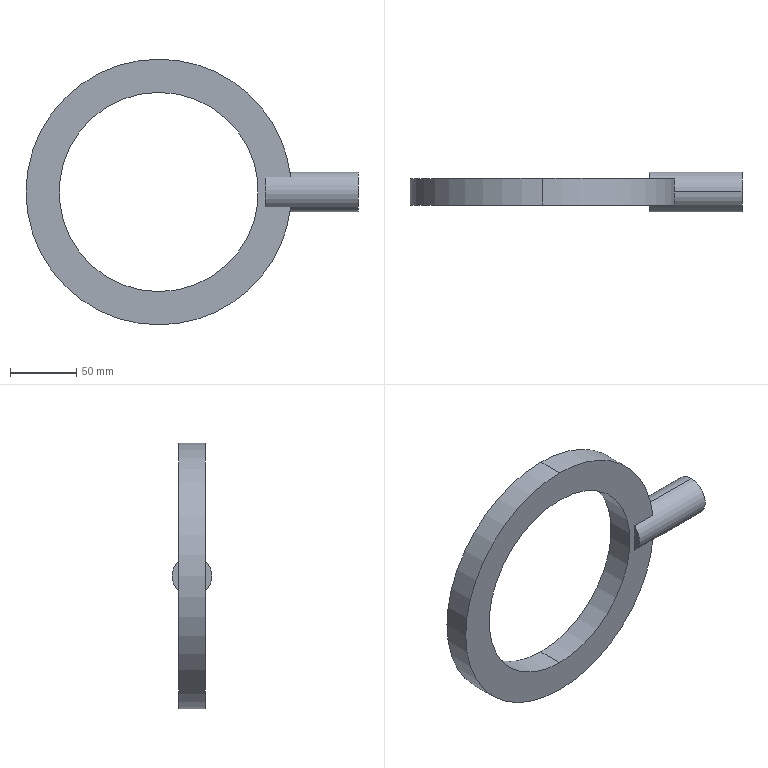Part | SolidWorks | features Extrusion 1, HoleWzd 1, ICE 1 | 1 solid | 16 faces | box 250 x 30 x 200 mm | volume 313165 mm3 | cylinder 9 | plane 5 | cone 2 | commonest cylinder face diameters 200 x3 5 x2 30 x2 150 x2
STEP:
#1=CARTESIAN_POINT('',(133.,10.,2.5));
#2=VERTEX_POINT('',#1);
#3=CARTESIAN_POINT('',(133.,10.,-2.5));
#4=VERTEX_POINT('',#3);
#5=CARTESIAN_POINT('',(133.,10.,0.));
#6=DIRECTION('',(1.,0.,0.));
#7=DIRECTION('',(0.,0.,-1.));
#8=AXIS2_PLACEMENT_3D('',#5,#6,#7);
#9=CIRCLE('',#8,2.5);
#10=EDGE_CURVE('',#2,#4,#9,.T.);
#11=ORIENTED_EDGE('',*,*,#10,.F.);
#12=CARTESIAN_POINT('',(150.,10.,2.5));
#13=VERTEX_POINT('',#12);
#14=CARTESIAN_POINT('',(150.,10.,2.5));
#15=DIRECTION('',(1.,0.,0.));
#16=VECTOR('',#15,1000.);
#17=LINE('',#14,#16);
#18=EDGE_CURVE('',#2,#13,#17,.T.);
#19=ORIENTED_EDGE('',*,*,#18,.T.);
#20=CARTESIAN_POINT('',(150.,10.,-2.5));
#21=VERTEX_POINT('',#20);
#22=CARTESIAN_POINT('',(150.,10.,0.));
#23=DIRECTION('',(1.,0.,0.));
#24=DIRECTION('',(0.,0.,-1.));
#25=AXIS2_PLACEMENT_3D('',#22,#23,#24);
#26=CIRCLE('',#25,2.5);
#27=EDGE_CURVE('',#13,#21,#26,.T.);
#28=ORIENTED_EDGE('',*,*,#27,.T.);
#29=CARTESIAN_POINT('',(150.,10.,-2.5));
#30=DIRECTION('',(1.,0.,0.));
#31=VECTOR('',#30,1000.);
#32=LINE('',#29,#31);
#33=EDGE_CURVE('',#4,#21,#32,.T.);
#34=ORIENTED_EDGE('',*,*,#33,.F.);
#35=EDGE_LOOP('',(#11,#19,#28,#34));
#36=FACE_OUTER_BOUND('',#35,.T.);
#37=CARTESIAN_POINT('',(150.,10.,0.));
#38=DIRECTION('',(1.,0.,0.));
#39=DIRECTION('',(0.,0.,-1.));
#40=AXIS2_PLACEMENT_3D('',#37,#38,#39);
#41=CYLINDRICAL_SURFACE('',#40,2.5);
#42=ADVANCED_FACE('',(#36),#41,.F.);
#43=CARTESIAN_POINT('',(131.498,10.,0.));
#44=VERTEX_POINT('',#43);
#45=CARTESIAN_POINT('',(133.,10.,-2.5));
#46=DIRECTION('',(0.515,0.,-0.8572));
#47=VECTOR('',#46,1000.);
#48=LINE('',#45,#47);
#49=EDGE_CURVE('',#44,#4,#48,.T.);
#50=ORIENTED_EDGE('',*,*,#49,.F.);
#51=CARTESIAN_POINT('',(133.,10.,2.5));
#52=DIRECTION('',(0.515,0.,0.8572));
#53=VECTOR('',#52,1000.);
#54=LINE('',#51,#53);
#55=EDGE_CURVE('',#44,#2,#54,.T.);
#56=ORIENTED_EDGE('',*,*,#55,.T.);
#57=ORIENTED_EDGE('',*,*,#10,.T.);
#58=EDGE_LOOP('',(#50,#56,#57));
#59=FACE_OUTER_BOUND('',#58,.T.);
#60=CARTESIAN_POINT('',(133.,10.,0.));
#61=DIRECTION('',(1.,0.,0.));
#62=DIRECTION('',(0.,0.,-1.));
#63=AXIS2_PLACEMENT_3D('',#60,#61,#62);
#64=CONICAL_SURFACE('',#63,2.5,1.03);
#65=ADVANCED_FACE('',(#59),#64,.F.);
#66=CARTESIAN_POINT('',(150.,10.,-15.));
#67=VERTEX_POINT('',#66);
#68=CARTESIAN_POINT('',(150.,10.,15.));
#69=VERTEX_POINT('',#68);
#70=CARTESIAN_POINT('',(150.,10.,0.));
#71=DIRECTION('',(1.,0.,0.));
#72=DIRECTION('',(0.,0.,-1.));
#73=AXIS2_PLACEMENT_3D('',#70,#71,#72);
#74=CIRCLE('',#73,15.);
#75=EDGE_CURVE('',#67,#69,#74,.T.);
#76=ORIENTED_EDGE('',*,*,#75,.F.);
#77=CARTESIAN_POINT('',(98.869,10.,-15.));
#78=VERTEX_POINT('',#77);
#79=CARTESIAN_POINT('',(150.,10.,-15.));
#80=DIRECTION('',(-1.,0.,0.));
#81=VECTOR('',#80,1000.);
#82=LINE('',#79,#81);
#83=EDGE_CURVE('',#67,#78,#82,.T.);
#84=ORIENTED_EDGE('',*,*,#83,.T.);
#85=CARTESIAN_POINT('',(99.373,20.,-11.18));
#86=VERTEX_POINT('',#85);
#87=CARTESIAN_POINT('',(98.869,10.,-15.));
#88=CARTESIAN_POINT('',(98.869,10.914,-15.));
#89=CARTESIAN_POINT('',(98.881,11.818,-14.917));
#90=CARTESIAN_POINT('',(98.918,13.161,-14.67));
#91=CARTESIAN_POINT('',(98.933,13.606,-14.567));
#92=CARTESIAN_POINT('',(98.97,14.492,-14.319));
#93=CARTESIAN_POINT('',(98.99,14.927,-14.175));
#94=CARTESIAN_POINT('',(99.059,16.202,-13.688));
#95=CARTESIAN_POINT('',(99.114,17.016,-13.289));
#96=CARTESIAN_POINT('',(99.206,18.184,-12.579));
#97=CARTESIAN_POINT('',(99.238,18.565,-12.323));
#98=CARTESIAN_POINT('',(99.305,19.302,-11.776));
#99=CARTESIAN_POINT('',(99.339,19.658,-11.487));
#100=CARTESIAN_POINT('',(99.373,20.,-11.18));
#101=B_SPLINE_CURVE_WITH_KNOTS('',3,(#87,#88,#89,#90,#91,#92,#93,#94,#95,#96,#97,#98,#99,#100),.UNSPECIFIED.,.F.,.F.,(4,2,2,2,2,2,4),(0.0109,0.01363,0.01499,0.01635,0.01908,0.02044,0.0218),.UNSPECIFIED.);
#102=EDGE_CURVE('',#78,#86,#101,.T.);
#103=ORIENTED_EDGE('',*,*,#102,.T.);
#104=CARTESIAN_POINT('',(80.,20.,-11.18));
#105=VERTEX_POINT('',#104);
#106=CARTESIAN_POINT('',(150.,20.,-11.18));
#107=DIRECTION('',(1.,0.,0.));
#108=VECTOR('',#107,1000.);
#109=LINE('',#106,#108);
#110=EDGE_CURVE('',#105,#86,#109,.T.);
#111=ORIENTED_EDGE('',*,*,#110,.F.);
#112=CARTESIAN_POINT('',(80.,20.,11.18));
#113=VERTEX_POINT('',#112);
#114=CARTESIAN_POINT('',(80.,10.,0.));
#115=DIRECTION('',(1.,0.,0.));
#116=DIRECTION('',(0.,0.,-1.));
#117=AXIS2_PLACEMENT_3D('',#114,#115,#116);
#118=CIRCLE('',#117,15.);
#119=EDGE_CURVE('',#105,#113,#118,.T.);
#120=ORIENTED_EDGE('',*,*,#119,.T.);
#121=CARTESIAN_POINT('',(99.373,20.,11.18));
#122=VERTEX_POINT('',#121);
#123=CARTESIAN_POINT('',(150.,20.,11.18));
#124=DIRECTION('',(-1.,0.,0.));
#125=VECTOR('',#124,1000.);
#126=LINE('',#123,#125);
#127=EDGE_CURVE('',#122,#113,#126,.T.);
#128=ORIENTED_EDGE('',*,*,#127,.F.);
#129=CARTESIAN_POINT('',(98.869,10.,15.));
#130=VERTEX_POINT('',#129);
#131=CARTESIAN_POINT('',(99.373,20.,11.18));
#132=CARTESIAN_POINT('',(99.304,19.315,11.793));
#133=CARTESIAN_POINT('',(99.238,18.584,12.334));
#134=CARTESIAN_POINT('',(99.146,17.423,13.042));
#135=CARTESIAN_POINT('',(99.117,17.025,13.261));
#136=CARTESIAN_POINT('',(99.062,16.207,13.663));
#137=CARTESIAN_POINT('',(99.037,15.784,13.848));
#138=CARTESIAN_POINT('',(98.967,14.5,14.339));
#139=CARTESIAN_POINT('',(98.931,13.624,14.584));
#140=CARTESIAN_POINT('',(98.894,12.284,14.832));
#141=CARTESIAN_POINT('',(98.885,11.832,14.895));
#142=CARTESIAN_POINT('',(98.872,10.919,14.979));
#143=CARTESIAN_POINT('',(98.869,10.457,15.));
#144=CARTESIAN_POINT('',(98.869,10.,15.));
#145=B_SPLINE_CURVE_WITH_KNOTS('',3,(#131,#132,#133,#134,#135,#136,#137,#138,#139,#140,#141,#142,#143,#144),.UNSPECIFIED.,.F.,.F.,(4,2,2,2,2,2,4),(0.,0.002726,0.004089,0.005452,0.008179,0.009542,0.0109),.UNSPECIFIED.);
#146=EDGE_CURVE('',#122,#130,#145,.T.);
#147=ORIENTED_EDGE('',*,*,#146,.T.);
#148=CARTESIAN_POINT('',(150.,10.,15.));
#149=DIRECTION('',(-1.,0.,0.));
#150=VECTOR('',#149,1000.);
#151=LINE('',#148,#150);
#152=EDGE_CURVE('',#69,#130,#151,.T.);
#153=ORIENTED_EDGE('',*,*,#152,.F.);
#154=EDGE_LOOP('',(#76,#84,#103,#111,#120,#128,#147,#153));
#155=FACE_OUTER_BOUND('',#154,.T.);
#156=CARTESIAN_POINT('',(150.,10.,0.));
#157=DIRECTION('',(-1.,0.,0.));
#158=DIRECTION('',(0.,0.,1.));
#159=AXIS2_PLACEMENT_3D('',#156,#157,#158);
#160=CYLINDRICAL_SURFACE('',#159,15.);
#161=ADVANCED_FACE('',(#155),#160,.T.);
#162=CARTESIAN_POINT('',(0.,20.,-75.));
#163=VERTEX_POINT('',#162);
#164=CARTESIAN_POINT('',(0.,20.,75.));
#165=VERTEX_POINT('',#164);
#166=CARTESIAN_POINT('',(0.,20.,0.));
#167=DIRECTION('',(0.,1.,0.));
#168=DIRECTION('',(0.,0.,1.));
#169=AXIS2_PLACEMENT_3D('',#166,#167,#168);
#170=CIRCLE('',#169,75.);
#171=EDGE_CURVE('',#163,#165,#170,.T.);
#172=ORIENTED_EDGE('',*,*,#171,.T.);
#173=CARTESIAN_POINT('',(0.,0.,75.));
#174=VERTEX_POINT('',#173);
#175=CARTESIAN_POINT('',(0.,20.,75.));
#176=DIRECTION('',(0.,-1.,0.));
#177=VECTOR('',#176,1000.);
#178=LINE('',#175,#177);
#179=EDGE_CURVE('',#165,#174,#178,.T.);
#180=ORIENTED_EDGE('',*,*,#179,.T.);
#181=CARTESIAN_POINT('',(0.,0.,-75.));
#182=VERTEX_POINT('',#181);
#183=CARTESIAN_POINT('',(0.,0.,0.));
#184=DIRECTION('',(0.,1.,0.));
#185=DIRECTION('',(0.,0.,1.));
#186=AXIS2_PLACEMENT_3D('',#183,#184,#185);
#187=CIRCLE('',#186,75.);
#188=EDGE_CURVE('',#182,#174,#187,.T.);
#189=ORIENTED_EDGE('',*,*,#188,.F.);
#190=CARTESIAN_POINT('',(0.,20.,-75.));
#191=DIRECTION('',(0.,-1.,0.));
#192=VECTOR('',#191,1000.);
#193=LINE('',#190,#192);
#194=EDGE_CURVE('',#163,#182,#193,.T.);
#195=ORIENTED_EDGE('',*,*,#194,.F.);
#196=EDGE_LOOP('',(#172,#180,#189,#195));
#197=FACE_OUTER_BOUND('',#196,.T.);
#198=CARTESIAN_POINT('',(0.,20.,0.));
#199=DIRECTION('',(0.,-1.,0.));
#200=DIRECTION('',(0.,0.,-1.));
#201=AXIS2_PLACEMENT_3D('',#198,#199,#200);
#202=CYLINDRICAL_SURFACE('',#201,75.);
#203=ADVANCED_FACE('',(#197),#202,.F.);
#204=CARTESIAN_POINT('',(0.,20.,100.));
#205=VERTEX_POINT('',#204);
#206=CARTESIAN_POINT('',(0.,20.,0.));
#207=DIRECTION('',(0.,1.,0.));
#208=DIRECTION('',(0.,0.,1.));
#209=AXIS2_PLACEMENT_3D('',#206,#207,#208);
#210=CIRCLE('',#209,100.);
#211=EDGE_CURVE('',#205,#122,#210,.T.);
#212=ORIENTED_EDGE('',*,*,#211,.F.);
#213=CARTESIAN_POINT('',(0.,0.,100.));
#214=VERTEX_POINT('',#213);
#215=CARTESIAN_POINT('',(0.,20.,100.));
#216=DIRECTION('',(0.,-1.,0.));
#217=VECTOR('',#216,1000.);
#218=LINE('',#215,#217);
#219=EDGE_CURVE('',#205,#214,#218,.T.);
#220=ORIENTED_EDGE('',*,*,#219,.T.);
#221=CARTESIAN_POINT('',(99.373,0.,11.18));
#222=VERTEX_POINT('',#221);
#223=CARTESIAN_POINT('',(0.,0.,0.));
#224=DIRECTION('',(0.,1.,0.));
#225=DIRECTION('',(0.,0.,1.));
#226=AXIS2_PLACEMENT_3D('',#223,#224,#225);
#227=CIRCLE('',#226,100.);
#228=EDGE_CURVE('',#214,#222,#227,.T.);
#229=ORIENTED_EDGE('',*,*,#228,.T.);
#230=CARTESIAN_POINT('',(98.869,10.,15.));
#231=CARTESIAN_POINT('',(98.869,9.086,15.));
#232=CARTESIAN_POINT('',(98.881,8.182,14.917));
#233=CARTESIAN_POINT('',(98.918,6.839,14.67));
#234=CARTESIAN_POINT('',(98.933,6.394,14.567));
#235=CARTESIAN_POINT('',(98.97,5.508,14.319));
#236=CARTESIAN_POINT('',(98.99,5.073,14.175));
#237=CARTESIAN_POINT('',(99.059,3.798,13.688));
#238=CARTESIAN_POINT('',(99.114,2.984,13.289));
#239=CARTESIAN_POINT('',(99.206,1.816,12.579));
#240=CARTESIAN_POINT('',(99.238,1.435,12.323));
#241=CARTESIAN_POINT('',(99.305,0.6978,11.776));
#242=CARTESIAN_POINT('',(99.339,0.3423,11.487));
#243=CARTESIAN_POINT('',(99.373,0.,11.18));
#244=B_SPLINE_CURVE_WITH_KNOTS('',3,(#230,#231,#232,#233,#234,#235,#236,#237,#238,#239,#240,#241,#242,#243),.UNSPECIFIED.,.F.,.F.,(4,2,2,2,2,2,4),(0.0109,0.01363,0.01499,0.01635,0.01908,0.02044,0.0218),.UNSPECIFIED.);
#245=EDGE_CURVE('',#130,#222,#244,.T.);
#246=ORIENTED_EDGE('',*,*,#245,.F.);
#247=ORIENTED_EDGE('',*,*,#146,.F.);
#248=EDGE_LOOP('',(#212,#220,#229,#246,#247));
#249=FACE_OUTER_BOUND('',#248,.T.);
#250=CARTESIAN_POINT('',(0.,20.,0.));
#251=DIRECTION('',(0.,-1.,0.));
#252=DIRECTION('',(0.,0.,-1.));
#253=AXIS2_PLACEMENT_3D('',#250,#251,#252);
#254=CYLINDRICAL_SURFACE('',#253,100.);
#255=ADVANCED_FACE('',(#249),#254,.T.);
#256=ORIENTED_EDGE('',*,*,#219,.F.);
#257=CARTESIAN_POINT('',(0.,20.,-100.));
#258=VERTEX_POINT('',#257);
#259=CARTESIAN_POINT('',(0.,20.,0.));
#260=DIRECTION('',(0.,1.,0.));
#261=DIRECTION('',(0.,0.,1.));
#262=AXIS2_PLACEMENT_3D('',#259,#260,#261);
#263=CIRCLE('',#262,100.);
#264=EDGE_CURVE('',#258,#205,#263,.T.);
#265=ORIENTED_EDGE('',*,*,#264,.F.);
#266=CARTESIAN_POINT('',(0.,0.,-100.));
#267=VERTEX_POINT('',#266);
#268=CARTESIAN_POINT('',(0.,20.,-100.));
#269=DIRECTION('',(0.,-1.,0.));
#270=VECTOR('',#269,1000.);
#271=LINE('',#268,#270);
#272=EDGE_CURVE('',#258,#267,#271,.T.);
#273=ORIENTED_EDGE('',*,*,#272,.T.);
#274=CARTESIAN_POINT('',(0.,0.,0.));
#275=DIRECTION('',(0.,1.,0.));
#276=DIRECTION('',(0.,0.,1.));
#277=AXIS2_PLACEMENT_3D('',#274,#275,#276);
#278=CIRCLE('',#277,100.);
#279=EDGE_CURVE('',#267,#214,#278,.T.);
#280=ORIENTED_EDGE('',*,*,#279,.T.);
#281=EDGE_LOOP('',(#256,#265,#273,#280));
#282=FACE_OUTER_BOUND('',#281,.T.);
#283=CARTESIAN_POINT('',(0.,20.,0.));
#284=DIRECTION('',(0.,-1.,0.));
#285=DIRECTION('',(0.,0.,-1.));
#286=AXIS2_PLACEMENT_3D('',#283,#284,#285);
#287=CYLINDRICAL_SURFACE('',#286,100.);
#288=ADVANCED_FACE('',(#282),#287,.T.);
#289=ORIENTED_EDGE('',*,*,#171,.F.);
#290=CARTESIAN_POINT('',(0.,20.,0.));
#291=DIRECTION('',(0.,1.,0.));
#292=DIRECTION('',(0.,0.,1.));
#293=AXIS2_PLACEMENT_3D('',#290,#291,#292);
#294=CIRCLE('',#293,75.);
#295=EDGE_CURVE('',#165,#163,#294,.T.);
#296=ORIENTED_EDGE('',*,*,#295,.F.);
#297=EDGE_LOOP('',(#289,#296));
#298=FACE_BOUND('',#297,.T.);
#299=CARTESIAN_POINT('',(80.,20.,0.));
#300=DIRECTION('',(0.,0.,-1.));
#301=VECTOR('',#300,1000.);
#302=LINE('',#299,#301);
#303=EDGE_CURVE('',#113,#105,#302,.T.);
#304=ORIENTED_EDGE('',*,*,#303,.T.);
#305=ORIENTED_EDGE('',*,*,#110,.T.);
#306=CARTESIAN_POINT('',(0.,20.,0.));
#307=DIRECTION('',(0.,1.,0.));
#308=DIRECTION('',(0.,0.,1.));
#309=AXIS2_PLACEMENT_3D('',#306,#307,#308);
#310=CIRCLE('',#309,100.);
#311=EDGE_CURVE('',#86,#258,#310,.T.);
#312=ORIENTED_EDGE('',*,*,#311,.T.);
#313=ORIENTED_EDGE('',*,*,#264,.T.);
#314=ORIENTED_EDGE('',*,*,#211,.T.);
#315=ORIENTED_EDGE('',*,*,#127,.T.);
#316=EDGE_LOOP('',(#304,#305,#312,#313,#314,#315));
#317=FACE_OUTER_BOUND('',#316,.T.);
#318=CARTESIAN_POINT('',(0.,20.,0.));
#319=DIRECTION('',(0.,1.,0.));
#320=DIRECTION('',(0.,0.,1.));
#321=AXIS2_PLACEMENT_3D('',#318,#319,#320);
#322=PLANE('',#321);
#323=ADVANCED_FACE('',(#298,#317),#322,.T.);
#324=ORIENTED_EDGE('',*,*,#188,.T.);
#325=CARTESIAN_POINT('',(0.,0.,0.));
#326=DIRECTION('',(0.,1.,0.));
#327=DIRECTION('',(0.,0.,1.));
#328=AXIS2_PLACEMENT_3D('',#325,#326,#327);
#329=CIRCLE('',#328,75.);
#330=EDGE_CURVE('',#174,#182,#329,.T.);
#331=ORIENTED_EDGE('',*,*,#330,.T.);
#332=EDGE_LOOP('',(#324,#331));
#333=FACE_BOUND('',#332,.T.);
#334=CARTESIAN_POINT('',(80.,0.,-11.18));
#335=VERTEX_POINT('',#334);
#336=CARTESIAN_POINT('',(99.373,0.,-11.18));
#337=VERTEX_POINT('',#336);
#338=CARTESIAN_POINT('',(150.,0.,-11.18));
#339=DIRECTION('',(1.,0.,0.));
#340=VECTOR('',#339,1000.);
#341=LINE('',#338,#340);
#342=EDGE_CURVE('',#335,#337,#341,.T.);
#343=ORIENTED_EDGE('',*,*,#342,.F.);
#344=CARTESIAN_POINT('',(80.,0.,11.18));
#345=VERTEX_POINT('',#344);
#346=CARTESIAN_POINT('',(80.,0.,0.));
#347=DIRECTION('',(0.,0.,-1.));
#348=VECTOR('',#347,1000.);
#349=LINE('',#346,#348);
#350=EDGE_CURVE('',#345,#335,#349,.T.);
#351=ORIENTED_EDGE('',*,*,#350,.F.);
#352=CARTESIAN_POINT('',(150.,0.,11.18));
#353=DIRECTION('',(-1.,0.,0.));
#354=VECTOR('',#353,1000.);
#355=LINE('',#352,#354);
#356=EDGE_CURVE('',#222,#345,#355,.T.);
#357=ORIENTED_EDGE('',*,*,#356,.F.);
#358=ORIENTED_EDGE('',*,*,#228,.F.);
#359=ORIENTED_EDGE('',*,*,#279,.F.);
#360=CARTESIAN_POINT('',(0.,0.,0.));
#361=DIRECTION('',(0.,1.,0.));
#362=DIRECTION('',(0.,0.,1.));
#363=AXIS2_PLACEMENT_3D('',#360,#361,#362);
#364=CIRCLE('',#363,100.);
#365=EDGE_CURVE('',#337,#267,#364,.T.);
#366=ORIENTED_EDGE('',*,*,#365,.F.);
#367=EDGE_LOOP('',(#343,#351,#357,#358,#359,#366));
#368=FACE_OUTER_BOUND('',#367,.T.);
#369=CARTESIAN_POINT('',(0.,0.,0.));
#370=DIRECTION('',(0.,1.,0.));
#371=DIRECTION('',(0.,0.,1.));
#372=AXIS2_PLACEMENT_3D('',#369,#370,#371);
#373=PLANE('',#372);
#374=ADVANCED_FACE('',(#333,#368),#373,.F.);
#375=ORIENTED_EDGE('',*,*,#272,.F.);
#376=ORIENTED_EDGE('',*,*,#311,.F.);
#377=ORIENTED_EDGE('',*,*,#102,.F.);
#378=CARTESIAN_POINT('',(99.373,0.,-11.18));
#379=CARTESIAN_POINT('',(99.304,0.6851,-11.793));
#380=CARTESIAN_POINT('',(99.238,1.416,-12.334));
#381=CARTESIAN_POINT('',(99.146,2.577,-13.042));
#382=CARTESIAN_POINT('',(99.117,2.975,-13.261));
#383=CARTESIAN_POINT('',(99.062,3.793,-13.663));
#384=CARTESIAN_POINT('',(99.037,4.216,-13.848));
#385=CARTESIAN_POINT('',(98.967,5.5,-14.339));
#386=CARTESIAN_POINT('',(98.931,6.376,-14.584));
#387=CARTESIAN_POINT('',(98.894,7.716,-14.832));
#388=CARTESIAN_POINT('',(98.885,8.168,-14.895));
#389=CARTESIAN_POINT('',(98.872,9.081,-14.979));
#390=CARTESIAN_POINT('',(98.869,9.543,-15.));
#391=CARTESIAN_POINT('',(98.869,10.,-15.));
#392=B_SPLINE_CURVE_WITH_KNOTS('',3,(#378,#379,#380,#381,#382,#383,#384,#385,#386,#387,#388,#389,#390,#391),.UNSPECIFIED.,.F.,.F.,(4,2,2,2,2,2,4),(0.,0.002726,0.004089,0.005452,0.008179,0.009542,0.0109),.UNSPECIFIED.);
#393=EDGE_CURVE('',#337,#78,#392,.T.);
#394=ORIENTED_EDGE('',*,*,#393,.F.);
#395=ORIENTED_EDGE('',*,*,#365,.T.);
#396=EDGE_LOOP('',(#375,#376,#377,#394,#395));
#397=FACE_OUTER_BOUND('',#396,.T.);
#398=CARTESIAN_POINT('',(0.,20.,0.));
#399=DIRECTION('',(0.,-1.,0.));
#400=DIRECTION('',(0.,0.,-1.));
#401=AXIS2_PLACEMENT_3D('',#398,#399,#400);
#402=CYLINDRICAL_SURFACE('',#401,100.);
#403=ADVANCED_FACE('',(#397),#402,.T.);
#404=ORIENTED_EDGE('',*,*,#179,.F.);
#405=ORIENTED_EDGE('',*,*,#295,.T.);
#406=ORIENTED_EDGE('',*,*,#194,.T.);
#407=ORIENTED_EDGE('',*,*,#330,.F.);
#408=EDGE_LOOP('',(#404,#405,#406,#407));
#409=FACE_OUTER_BOUND('',#408,.T.);
#410=CARTESIAN_POINT('',(0.,20.,0.));
#411=DIRECTION('',(0.,-1.,0.));
#412=DIRECTION('',(0.,0.,-1.));
#413=AXIS2_PLACEMENT_3D('',#410,#411,#412);
#414=CYLINDRICAL_SURFACE('',#413,75.);
#415=ADVANCED_FACE('',(#409),#414,.F.);
#416=CARTESIAN_POINT('',(80.,10.,0.));
#417=DIRECTION('',(1.,0.,0.));
#418=DIRECTION('',(0.,0.,-1.));
#419=AXIS2_PLACEMENT_3D('',#416,#417,#418);
#420=CIRCLE('',#419,15.);
#421=EDGE_CURVE('',#345,#335,#420,.T.);
#422=ORIENTED_EDGE('',*,*,#421,.F.);
#423=ORIENTED_EDGE('',*,*,#350,.T.);
#424=EDGE_LOOP('',(#422,#423));
#425=FACE_OUTER_BOUND('',#424,.T.);
#426=CARTESIAN_POINT('',(80.,10.,0.));
#427=DIRECTION('',(1.,0.,0.));
#428=DIRECTION('',(0.,0.,-1.));
#429=AXIS2_PLACEMENT_3D('',#426,#427,#428);
#430=PLANE('',#429);
#431=ADVANCED_FACE('',(#425),#430,.F.);
#432=ORIENTED_EDGE('',*,*,#83,.F.);
#433=CARTESIAN_POINT('',(150.,10.,0.));
#434=DIRECTION('',(1.,0.,0.));
#435=DIRECTION('',(0.,0.,-1.));
#436=AXIS2_PLACEMENT_3D('',#433,#434,#435);
#437=CIRCLE('',#436,15.);
#438=EDGE_CURVE('',#69,#67,#437,.T.);
#439=ORIENTED_EDGE('',*,*,#438,.F.);
#440=ORIENTED_EDGE('',*,*,#152,.T.);
#441=ORIENTED_EDGE('',*,*,#245,.T.);
#442=ORIENTED_EDGE('',*,*,#356,.T.);
#443=ORIENTED_EDGE('',*,*,#421,.T.);
#444=ORIENTED_EDGE('',*,*,#342,.T.);
#445=ORIENTED_EDGE('',*,*,#393,.T.);
#446=EDGE_LOOP('',(#432,#439,#440,#441,#442,#443,#444,#445));
#447=FACE_OUTER_BOUND('',#446,.T.);
#448=CARTESIAN_POINT('',(150.,10.,0.));
#449=DIRECTION('',(-1.,0.,0.));
#450=DIRECTION('',(0.,0.,1.));
#451=AXIS2_PLACEMENT_3D('',#448,#449,#450);
#452=CYLINDRICAL_SURFACE('',#451,15.);
#453=ADVANCED_FACE('',(#447),#452,.T.);
#454=CARTESIAN_POINT('',(150.,10.,0.));
#455=DIRECTION('',(1.,0.,0.));
#456=DIRECTION('',(0.,0.,-1.));
#457=AXIS2_PLACEMENT_3D('',#454,#455,#456);
#458=CIRCLE('',#457,2.5);
#459=EDGE_CURVE('',#21,#13,#458,.T.);
#460=ORIENTED_EDGE('',*,*,#459,.F.);
#461=ORIENTED_EDGE('',*,*,#27,.F.);
#462=EDGE_LOOP('',(#460,#461));
#463=FACE_BOUND('',#462,.T.);
#464=ORIENTED_EDGE('',*,*,#438,.T.);
#465=ORIENTED_EDGE('',*,*,#75,.T.);
#466=EDGE_LOOP('',(#464,#465));
#467=FACE_OUTER_BOUND('',#466,.T.);
#468=CARTESIAN_POINT('',(150.,10.,0.));
#469=DIRECTION('',(1.,0.,0.));
#470=DIRECTION('',(0.,0.,-1.));
#471=AXIS2_PLACEMENT_3D('',#468,#469,#470);
#472=PLANE('',#471);
#473=ADVANCED_FACE('',(#463,#467),#472,.T.);
#474=ORIENTED_EDGE('',*,*,#303,.F.);
#475=ORIENTED_EDGE('',*,*,#119,.F.);
#476=EDGE_LOOP('',(#474,#475));
#477=FACE_OUTER_BOUND('',#476,.T.);
#478=CARTESIAN_POINT('',(80.,10.,0.));
#479=DIRECTION('',(1.,0.,0.));
#480=DIRECTION('',(0.,0.,-1.));
#481=AXIS2_PLACEMENT_3D('',#478,#479,#480);
#482=PLANE('',#481);
#483=ADVANCED_FACE('',(#477),#482,.F.);
#484=ORIENTED_EDGE('',*,*,#55,.F.);
#485=ORIENTED_EDGE('',*,*,#49,.T.);
#486=CARTESIAN_POINT('',(133.,10.,0.));
#487=DIRECTION('',(1.,0.,0.));
#488=DIRECTION('',(0.,0.,-1.));
#489=AXIS2_PLACEMENT_3D('',#486,#487,#488);
#490=CIRCLE('',#489,2.5);
#491=EDGE_CURVE('',#4,#2,#490,.T.);
#492=ORIENTED_EDGE('',*,*,#491,.T.);
#493=EDGE_LOOP('',(#484,#485,#492));
#494=FACE_OUTER_BOUND('',#493,.T.);
#495=CARTESIAN_POINT('',(133.,10.,0.));
#496=DIRECTION('',(1.,0.,0.));
#497=DIRECTION('',(0.,0.,-1.));
#498=AXIS2_PLACEMENT_3D('',#495,#496,#497);
#499=CONICAL_SURFACE('',#498,2.5,1.03);
#500=ADVANCED_FACE('',(#494),#499,.F.);
#501=ORIENTED_EDGE('',*,*,#18,.F.);
#502=ORIENTED_EDGE('',*,*,#491,.F.);
#503=ORIENTED_EDGE('',*,*,#33,.T.);
#504=ORIENTED_EDGE('',*,*,#459,.T.);
#505=EDGE_LOOP('',(#501,#502,#503,#504));
#506=FACE_OUTER_BOUND('',#505,.T.);
#507=CARTESIAN_POINT('',(150.,10.,0.));
#508=DIRECTION('',(1.,0.,0.));
#509=DIRECTION('',(0.,0.,-1.));
#510=AXIS2_PLACEMENT_3D('',#507,#508,#509);
#511=CYLINDRICAL_SURFACE('',#510,2.5);
#512=ADVANCED_FACE('',(#506),#511,.F.);
#513=CLOSED_SHELL('',(#42,#65,#161,#203,#255,#288,#323,#374,#403,#415,#431,#453,#473,#483,#500,#512));
#514=MANIFOLD_SOLID_BREP('',#513);
#515=CARTESIAN_POINT('',(0.,0.,0.));
#516=DIRECTION('',(0.,0.,1.));
#517=DIRECTION('',(1.,0.,0.));
#518=AXIS2_PLACEMENT_3D('',#515,#516,#517);
#519=(LENGTH_UNIT()NAMED_UNIT(*)SI_UNIT(.MILLI.,.METRE.));
#520=UNCERTAINTY_MEASURE_WITH_UNIT(LENGTH_MEASURE(0.00001),#519,'','');
#521=(NAMED_UNIT(*)PLANE_ANGLE_UNIT()SI_UNIT($,.RADIAN.));
#522=(NAMED_UNIT(*)SI_UNIT($,.STERADIAN.)SOLID_ANGLE_UNIT());
#523=(GEOMETRIC_REPRESENTATION_CONTEXT(3)GLOBAL_UNCERTAINTY_ASSIGNED_CONTEXT((#520))GLOBAL_UNIT_ASSIGNED_CONTEXT((#519,#521,#522))REPRESENTATION_CONTEXT('',''));
#524=ADVANCED_BREP_SHAPE_REPRESENTATION('',(#514,#518),#523);